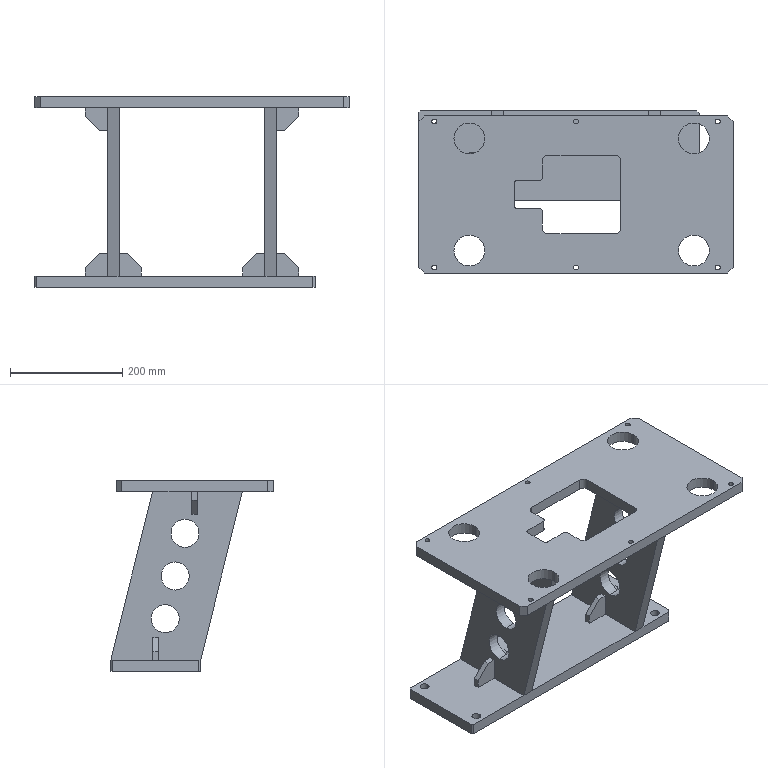Part | STEP file | Lifting Bracket | 1 solid | 116 faces | box 560 x 289.5 x 340 mm | volume 5840696 mm3 | plane 68 | cylinder 48 | commonest cylinder face diameters 8.5 x12 50 x12 15.5 x8 55 x8 10 x4 20 x4